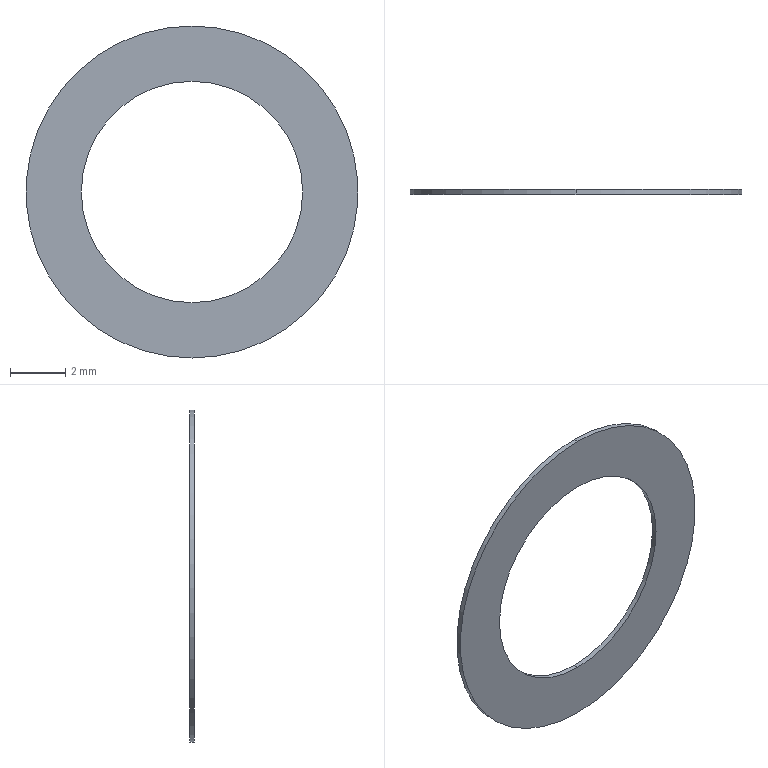Part | SolidWorks | features BaseBody 1 | 1 solid | 6 faces | box 12 x 0.18 x 12 mm | volume 11.31 mm3 | cylinder 4 | plane 2 | commonest cylinder face diameters 8 x2 12 x2
STEP:
#1=CARTESIAN_POINT('',(0.,0.18,4.));
#2=VERTEX_POINT('',#1);
#3=CARTESIAN_POINT('',(0.,0.,4.));
#4=VERTEX_POINT('',#3);
#5=CARTESIAN_POINT('',(0.,0.18,4.));
#6=DIRECTION('',(0.,-1.,0.));
#7=VECTOR('',#6,1000.);
#8=LINE('',#5,#7);
#9=EDGE_CURVE('',#2,#4,#8,.T.);
#10=ORIENTED_EDGE('',*,*,#9,.F.);
#11=CARTESIAN_POINT('',(0.,0.18,-4.));
#12=VERTEX_POINT('',#11);
#13=CARTESIAN_POINT('',(0.,0.18,0.));
#14=DIRECTION('',(0.,1.,0.));
#15=DIRECTION('',(0.,0.,1.));
#16=AXIS2_PLACEMENT_3D('',#13,#14,#15);
#17=CIRCLE('',#16,4.);
#18=EDGE_CURVE('',#2,#12,#17,.T.);
#19=ORIENTED_EDGE('',*,*,#18,.T.);
#20=CARTESIAN_POINT('',(0.,0.,-4.));
#21=VERTEX_POINT('',#20);
#22=CARTESIAN_POINT('',(0.,0.18,-4.));
#23=DIRECTION('',(0.,-1.,0.));
#24=VECTOR('',#23,1000.);
#25=LINE('',#22,#24);
#26=EDGE_CURVE('',#12,#21,#25,.T.);
#27=ORIENTED_EDGE('',*,*,#26,.T.);
#28=CARTESIAN_POINT('',(0.,0.,0.));
#29=DIRECTION('',(0.,1.,0.));
#30=DIRECTION('',(0.,0.,1.));
#31=AXIS2_PLACEMENT_3D('',#28,#29,#30);
#32=CIRCLE('',#31,4.);
#33=EDGE_CURVE('',#4,#21,#32,.T.);
#34=ORIENTED_EDGE('',*,*,#33,.F.);
#35=EDGE_LOOP('',(#10,#19,#27,#34));
#36=FACE_OUTER_BOUND('',#35,.T.);
#37=CARTESIAN_POINT('',(0.,0.18,0.));
#38=DIRECTION('',(0.,-1.,0.));
#39=DIRECTION('',(0.,0.,-1.));
#40=AXIS2_PLACEMENT_3D('',#37,#38,#39);
#41=CYLINDRICAL_SURFACE('',#40,4.);
#42=ADVANCED_FACE('',(#36),#41,.F.);
#43=CARTESIAN_POINT('',(0.,0.18,6.));
#44=VERTEX_POINT('',#43);
#45=CARTESIAN_POINT('',(0.,0.,6.));
#46=VERTEX_POINT('',#45);
#47=CARTESIAN_POINT('',(0.,0.18,6.));
#48=DIRECTION('',(0.,-1.,0.));
#49=VECTOR('',#48,1000.);
#50=LINE('',#47,#49);
#51=EDGE_CURVE('',#44,#46,#50,.T.);
#52=ORIENTED_EDGE('',*,*,#51,.F.);
#53=CARTESIAN_POINT('',(0.,0.18,-6.));
#54=VERTEX_POINT('',#53);
#55=CARTESIAN_POINT('',(0.,0.18,0.));
#56=DIRECTION('',(0.,1.,0.));
#57=DIRECTION('',(0.,0.,1.));
#58=AXIS2_PLACEMENT_3D('',#55,#56,#57);
#59=CIRCLE('',#58,6.);
#60=EDGE_CURVE('',#54,#44,#59,.T.);
#61=ORIENTED_EDGE('',*,*,#60,.F.);
#62=CARTESIAN_POINT('',(0.,0.,-6.));
#63=VERTEX_POINT('',#62);
#64=CARTESIAN_POINT('',(0.,0.18,-6.));
#65=DIRECTION('',(0.,-1.,0.));
#66=VECTOR('',#65,1000.);
#67=LINE('',#64,#66);
#68=EDGE_CURVE('',#54,#63,#67,.T.);
#69=ORIENTED_EDGE('',*,*,#68,.T.);
#70=CARTESIAN_POINT('',(0.,0.,0.));
#71=DIRECTION('',(0.,1.,0.));
#72=DIRECTION('',(0.,0.,1.));
#73=AXIS2_PLACEMENT_3D('',#70,#71,#72);
#74=CIRCLE('',#73,6.);
#75=EDGE_CURVE('',#63,#46,#74,.T.);
#76=ORIENTED_EDGE('',*,*,#75,.T.);
#77=EDGE_LOOP('',(#52,#61,#69,#76));
#78=FACE_OUTER_BOUND('',#77,.T.);
#79=CARTESIAN_POINT('',(0.,0.18,0.));
#80=DIRECTION('',(0.,-1.,0.));
#81=DIRECTION('',(0.,0.,-1.));
#82=AXIS2_PLACEMENT_3D('',#79,#80,#81);
#83=CYLINDRICAL_SURFACE('',#82,6.);
#84=ADVANCED_FACE('',(#78),#83,.T.);
#85=CARTESIAN_POINT('',(0.,0.,0.));
#86=DIRECTION('',(0.,1.,0.));
#87=DIRECTION('',(0.,0.,1.));
#88=AXIS2_PLACEMENT_3D('',#85,#86,#87);
#89=CIRCLE('',#88,4.);
#90=EDGE_CURVE('',#21,#4,#89,.T.);
#91=ORIENTED_EDGE('',*,*,#90,.T.);
#92=ORIENTED_EDGE('',*,*,#33,.T.);
#93=EDGE_LOOP('',(#91,#92));
#94=FACE_BOUND('',#93,.T.);
#95=ORIENTED_EDGE('',*,*,#75,.F.);
#96=CARTESIAN_POINT('',(0.,0.,0.));
#97=DIRECTION('',(0.,1.,0.));
#98=DIRECTION('',(0.,0.,1.));
#99=AXIS2_PLACEMENT_3D('',#96,#97,#98);
#100=CIRCLE('',#99,6.);
#101=EDGE_CURVE('',#46,#63,#100,.T.);
#102=ORIENTED_EDGE('',*,*,#101,.F.);
#103=EDGE_LOOP('',(#95,#102));
#104=FACE_OUTER_BOUND('',#103,.T.);
#105=CARTESIAN_POINT('',(0.,0.,0.));
#106=DIRECTION('',(0.,1.,0.));
#107=DIRECTION('',(1.,0.,0.));
#108=AXIS2_PLACEMENT_3D('',#105,#106,#107);
#109=PLANE('',#108);
#110=ADVANCED_FACE('',(#94,#104),#109,.F.);
#111=CARTESIAN_POINT('',(0.,0.18,0.));
#112=DIRECTION('',(0.,1.,0.));
#113=DIRECTION('',(0.,0.,1.));
#114=AXIS2_PLACEMENT_3D('',#111,#112,#113);
#115=CIRCLE('',#114,4.);
#116=EDGE_CURVE('',#12,#2,#115,.T.);
#117=ORIENTED_EDGE('',*,*,#116,.F.);
#118=ORIENTED_EDGE('',*,*,#18,.F.);
#119=EDGE_LOOP('',(#117,#118));
#120=FACE_BOUND('',#119,.T.);
#121=ORIENTED_EDGE('',*,*,#60,.T.);
#122=CARTESIAN_POINT('',(0.,0.18,0.));
#123=DIRECTION('',(0.,1.,0.));
#124=DIRECTION('',(0.,0.,1.));
#125=AXIS2_PLACEMENT_3D('',#122,#123,#124);
#126=CIRCLE('',#125,6.);
#127=EDGE_CURVE('',#44,#54,#126,.T.);
#128=ORIENTED_EDGE('',*,*,#127,.T.);
#129=EDGE_LOOP('',(#121,#128));
#130=FACE_OUTER_BOUND('',#129,.T.);
#131=CARTESIAN_POINT('',(0.,0.18,0.));
#132=DIRECTION('',(0.,1.,0.));
#133=DIRECTION('',(1.,0.,0.));
#134=AXIS2_PLACEMENT_3D('',#131,#132,#133);
#135=PLANE('',#134);
#136=ADVANCED_FACE('',(#120,#130),#135,.T.);
#137=ORIENTED_EDGE('',*,*,#127,.F.);
#138=ORIENTED_EDGE('',*,*,#51,.T.);
#139=ORIENTED_EDGE('',*,*,#101,.T.);
#140=ORIENTED_EDGE('',*,*,#68,.F.);
#141=EDGE_LOOP('',(#137,#138,#139,#140));
#142=FACE_OUTER_BOUND('',#141,.T.);
#143=CARTESIAN_POINT('',(0.,0.18,0.));
#144=DIRECTION('',(0.,-1.,0.));
#145=DIRECTION('',(0.,0.,-1.));
#146=AXIS2_PLACEMENT_3D('',#143,#144,#145);
#147=CYLINDRICAL_SURFACE('',#146,6.);
#148=ADVANCED_FACE('',(#142),#147,.T.);
#149=ORIENTED_EDGE('',*,*,#116,.T.);
#150=ORIENTED_EDGE('',*,*,#9,.T.);
#151=ORIENTED_EDGE('',*,*,#90,.F.);
#152=ORIENTED_EDGE('',*,*,#26,.F.);
#153=EDGE_LOOP('',(#149,#150,#151,#152));
#154=FACE_OUTER_BOUND('',#153,.T.);
#155=CARTESIAN_POINT('',(0.,0.18,0.));
#156=DIRECTION('',(0.,-1.,0.));
#157=DIRECTION('',(0.,0.,-1.));
#158=AXIS2_PLACEMENT_3D('',#155,#156,#157);
#159=CYLINDRICAL_SURFACE('',#158,4.);
#160=ADVANCED_FACE('',(#154),#159,.F.);
#161=CLOSED_SHELL('',(#42,#84,#110,#136,#148,#160));
#162=MANIFOLD_SOLID_BREP('',#161);
#163=CARTESIAN_POINT('',(0.,0.,0.));
#164=DIRECTION('',(0.,0.,1.));
#165=DIRECTION('',(1.,0.,0.));
#166=AXIS2_PLACEMENT_3D('',#163,#164,#165);
#167=(LENGTH_UNIT()NAMED_UNIT(*)SI_UNIT(.MILLI.,.METRE.));
#168=UNCERTAINTY_MEASURE_WITH_UNIT(LENGTH_MEASURE(0.00001),#167,'','');
#169=(NAMED_UNIT(*)PLANE_ANGLE_UNIT()SI_UNIT($,.RADIAN.));
#170=(NAMED_UNIT(*)SI_UNIT($,.STERADIAN.)SOLID_ANGLE_UNIT());
#171=(GEOMETRIC_REPRESENTATION_CONTEXT(3)GLOBAL_UNCERTAINTY_ASSIGNED_CONTEXT((#168))GLOBAL_UNIT_ASSIGNED_CONTEXT((#167,#169,#170))REPRESENTATION_CONTEXT('',''));
#172=ADVANCED_BREP_SHAPE_REPRESENTATION('',(#162,#166),#171);